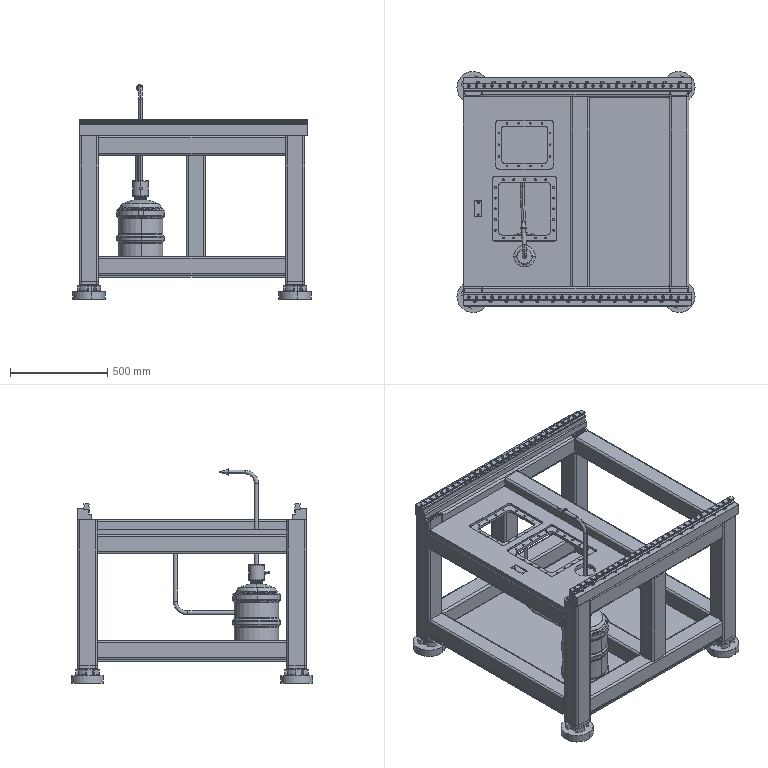Part | SolidWorks | 43 solids | 2257 faces | box 1225 x 1241 x 1104 mm | volume 76419257 mm3 | cylinder 913 | plane 699 | spline 399 | cone 160 | torus 82 | sphere 4 | commonest cylinder face diameters 6.5 x148 14 x132 9 x116 20 x104 16 x72 2 x64